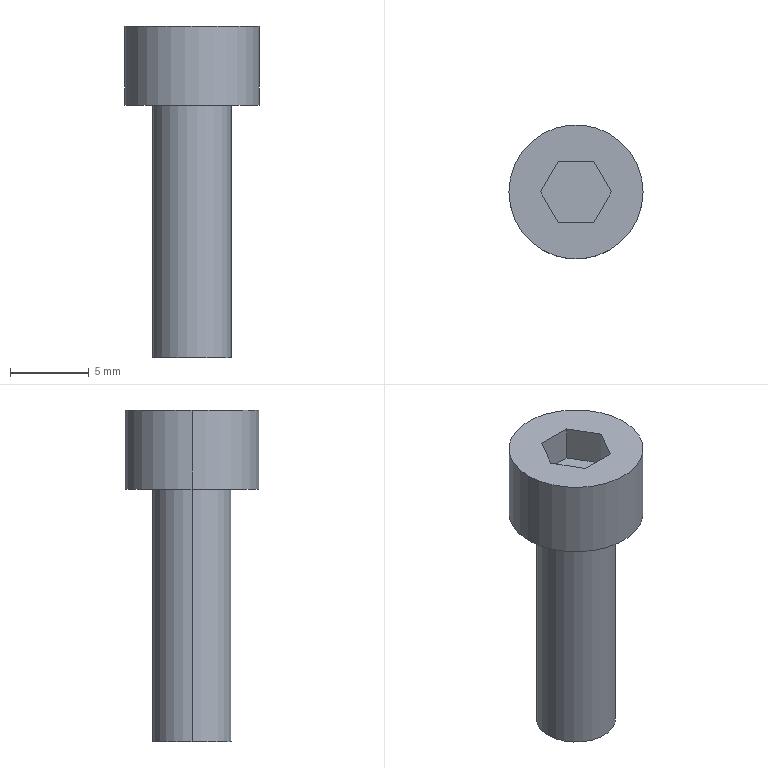Part | SolidWorks | features BaseBody 1 | 1 solid | 14 faces | box 8.5 x 8.5 x 21 mm | volume 568.291 mm3 | plane 10 | cylinder 4 | commonest cylinder face diameters 5 x2 8.5 x2
STEP:
#1=CARTESIAN_POINT('',(2.5,0.,-16.));
#2=VERTEX_POINT('',#1);
#3=CARTESIAN_POINT('',(-2.5,0.,-16.));
#4=VERTEX_POINT('',#3);
#5=CARTESIAN_POINT('',(0.,0.,-16.));
#6=DIRECTION('',(0.,0.,1.));
#7=DIRECTION('',(1.,0.,0.));
#8=AXIS2_PLACEMENT_3D('',#5,#6,#7);
#9=CIRCLE('',#8,2.5);
#10=EDGE_CURVE('',#2,#4,#9,.T.);
#11=ORIENTED_EDGE('',*,*,#10,.T.);
#12=CARTESIAN_POINT('',(-2.5,0.,0.));
#13=VERTEX_POINT('',#12);
#14=CARTESIAN_POINT('',(-2.5,0.,-16.));
#15=DIRECTION('',(0.,0.,1.));
#16=VECTOR('',#15,1000.);
#17=LINE('',#14,#16);
#18=EDGE_CURVE('',#4,#13,#17,.T.);
#19=ORIENTED_EDGE('',*,*,#18,.T.);
#20=CARTESIAN_POINT('',(2.5,0.,0.));
#21=VERTEX_POINT('',#20);
#22=CARTESIAN_POINT('',(0.,0.,0.));
#23=DIRECTION('',(0.,0.,-1.));
#24=DIRECTION('',(1.,0.,0.));
#25=AXIS2_PLACEMENT_3D('',#22,#23,#24);
#26=CIRCLE('',#25,2.5);
#27=EDGE_CURVE('',#13,#21,#26,.T.);
#28=ORIENTED_EDGE('',*,*,#27,.T.);
#29=CARTESIAN_POINT('',(2.5,0.,-16.));
#30=DIRECTION('',(0.,0.,1.));
#31=VECTOR('',#30,1000.);
#32=LINE('',#29,#31);
#33=EDGE_CURVE('',#2,#21,#32,.T.);
#34=ORIENTED_EDGE('',*,*,#33,.F.);
#35=EDGE_LOOP('',(#11,#19,#28,#34));
#36=FACE_OUTER_BOUND('',#35,.T.);
#37=CARTESIAN_POINT('',(0.,0.,-16.));
#38=DIRECTION('',(0.,0.,1.));
#39=DIRECTION('',(1.,0.,0.));
#40=AXIS2_PLACEMENT_3D('',#37,#38,#39);
#41=CYLINDRICAL_SURFACE('',#40,2.5);
#42=ADVANCED_FACE('',(#36),#41,.T.);
#43=CARTESIAN_POINT('',(4.25,0.,0.));
#44=VERTEX_POINT('',#43);
#45=CARTESIAN_POINT('',(-4.25,0.,0.));
#46=VERTEX_POINT('',#45);
#47=CARTESIAN_POINT('',(0.,0.,0.));
#48=DIRECTION('',(0.,0.,1.));
#49=DIRECTION('',(1.,0.,0.));
#50=AXIS2_PLACEMENT_3D('',#47,#48,#49);
#51=CIRCLE('',#50,4.25);
#52=EDGE_CURVE('',#44,#46,#51,.T.);
#53=ORIENTED_EDGE('',*,*,#52,.T.);
#54=CARTESIAN_POINT('',(-4.25,0.,5.));
#55=VERTEX_POINT('',#54);
#56=CARTESIAN_POINT('',(-4.25,0.,0.));
#57=DIRECTION('',(0.,0.,1.));
#58=VECTOR('',#57,1000.);
#59=LINE('',#56,#58);
#60=EDGE_CURVE('',#46,#55,#59,.T.);
#61=ORIENTED_EDGE('',*,*,#60,.T.);
#62=CARTESIAN_POINT('',(4.25,0.,5.));
#63=VERTEX_POINT('',#62);
#64=CARTESIAN_POINT('',(0.,0.,5.));
#65=DIRECTION('',(0.,0.,-1.));
#66=DIRECTION('',(1.,0.,0.));
#67=AXIS2_PLACEMENT_3D('',#64,#65,#66);
#68=CIRCLE('',#67,4.25);
#69=EDGE_CURVE('',#55,#63,#68,.T.);
#70=ORIENTED_EDGE('',*,*,#69,.T.);
#71=CARTESIAN_POINT('',(4.25,0.,0.));
#72=DIRECTION('',(0.,0.,1.));
#73=VECTOR('',#72,1000.);
#74=LINE('',#71,#73);
#75=EDGE_CURVE('',#44,#63,#74,.T.);
#76=ORIENTED_EDGE('',*,*,#75,.F.);
#77=EDGE_LOOP('',(#53,#61,#70,#76));
#78=FACE_OUTER_BOUND('',#77,.T.);
#79=CARTESIAN_POINT('',(0.,0.,0.));
#80=DIRECTION('',(0.,0.,1.));
#81=DIRECTION('',(1.,0.,0.));
#82=AXIS2_PLACEMENT_3D('',#79,#80,#81);
#83=CYLINDRICAL_SURFACE('',#82,4.25);
#84=ADVANCED_FACE('',(#78),#83,.T.);
#85=ORIENTED_EDGE('',*,*,#18,.F.);
#86=CARTESIAN_POINT('',(0.,0.,-16.));
#87=DIRECTION('',(0.,0.,1.));
#88=DIRECTION('',(1.,0.,0.));
#89=AXIS2_PLACEMENT_3D('',#86,#87,#88);
#90=CIRCLE('',#89,2.5);
#91=EDGE_CURVE('',#4,#2,#90,.T.);
#92=ORIENTED_EDGE('',*,*,#91,.T.);
#93=ORIENTED_EDGE('',*,*,#33,.T.);
#94=CARTESIAN_POINT('',(0.,0.,0.));
#95=DIRECTION('',(0.,0.,-1.));
#96=DIRECTION('',(1.,0.,0.));
#97=AXIS2_PLACEMENT_3D('',#94,#95,#96);
#98=CIRCLE('',#97,2.5);
#99=EDGE_CURVE('',#21,#13,#98,.T.);
#100=ORIENTED_EDGE('',*,*,#99,.T.);
#101=EDGE_LOOP('',(#85,#92,#93,#100));
#102=FACE_OUTER_BOUND('',#101,.T.);
#103=CARTESIAN_POINT('',(0.,0.,-16.));
#104=DIRECTION('',(0.,0.,1.));
#105=DIRECTION('',(1.,0.,0.));
#106=AXIS2_PLACEMENT_3D('',#103,#104,#105);
#107=CYLINDRICAL_SURFACE('',#106,2.5);
#108=ADVANCED_FACE('',(#102),#107,.T.);
#109=ORIENTED_EDGE('',*,*,#10,.F.);
#110=ORIENTED_EDGE('',*,*,#91,.F.);
#111=EDGE_LOOP('',(#109,#110));
#112=FACE_OUTER_BOUND('',#111,.T.);
#113=CARTESIAN_POINT('',(0.,0.,-16.));
#114=DIRECTION('',(0.,0.,1.));
#115=DIRECTION('',(1.,0.,0.));
#116=AXIS2_PLACEMENT_3D('',#113,#114,#115);
#117=PLANE('',#116);
#118=ADVANCED_FACE('',(#112),#117,.F.);
#119=ORIENTED_EDGE('',*,*,#99,.F.);
#120=ORIENTED_EDGE('',*,*,#27,.F.);
#121=EDGE_LOOP('',(#119,#120));
#122=FACE_BOUND('',#121,.T.);
#123=ORIENTED_EDGE('',*,*,#52,.F.);
#124=CARTESIAN_POINT('',(0.,0.,0.));
#125=DIRECTION('',(0.,0.,1.));
#126=DIRECTION('',(1.,0.,0.));
#127=AXIS2_PLACEMENT_3D('',#124,#125,#126);
#128=CIRCLE('',#127,4.25);
#129=EDGE_CURVE('',#46,#44,#128,.T.);
#130=ORIENTED_EDGE('',*,*,#129,.F.);
#131=EDGE_LOOP('',(#123,#130));
#132=FACE_OUTER_BOUND('',#131,.T.);
#133=CARTESIAN_POINT('',(0.,0.,0.));
#134=DIRECTION('',(0.,0.,1.));
#135=DIRECTION('',(1.,0.,0.));
#136=AXIS2_PLACEMENT_3D('',#133,#134,#135);
#137=PLANE('',#136);
#138=ADVANCED_FACE('',(#122,#132),#137,.F.);
#139=ORIENTED_EDGE('',*,*,#60,.F.);
#140=ORIENTED_EDGE('',*,*,#129,.T.);
#141=ORIENTED_EDGE('',*,*,#75,.T.);
#142=CARTESIAN_POINT('',(0.,0.,5.));
#143=DIRECTION('',(0.,0.,-1.));
#144=DIRECTION('',(1.,0.,0.));
#145=AXIS2_PLACEMENT_3D('',#142,#143,#144);
#146=CIRCLE('',#145,4.25);
#147=EDGE_CURVE('',#63,#55,#146,.T.);
#148=ORIENTED_EDGE('',*,*,#147,.T.);
#149=EDGE_LOOP('',(#139,#140,#141,#148));
#150=FACE_OUTER_BOUND('',#149,.T.);
#151=CARTESIAN_POINT('',(0.,0.,0.));
#152=DIRECTION('',(0.,0.,1.));
#153=DIRECTION('',(1.,0.,0.));
#154=AXIS2_PLACEMENT_3D('',#151,#152,#153);
#155=CYLINDRICAL_SURFACE('',#154,4.25);
#156=ADVANCED_FACE('',(#150),#155,.T.);
#157=CARTESIAN_POINT('',(-1.125,-1.949,5.));
#158=VERTEX_POINT('',#157);
#159=CARTESIAN_POINT('',(-2.25,0.,5.));
#160=VERTEX_POINT('',#159);
#161=CARTESIAN_POINT('',(-1.125,-1.949,5.));
#162=DIRECTION('',(-0.5,0.866,0.));
#163=VECTOR('',#162,1000.);
#164=LINE('',#161,#163);
#165=EDGE_CURVE('',#158,#160,#164,.T.);
#166=ORIENTED_EDGE('',*,*,#165,.T.);
#167=CARTESIAN_POINT('',(-1.125,1.949,5.));
#168=VERTEX_POINT('',#167);
#169=CARTESIAN_POINT('',(-2.25,0.,5.));
#170=DIRECTION('',(0.5,0.866,0.));
#171=VECTOR('',#170,1000.);
#172=LINE('',#169,#171);
#173=EDGE_CURVE('',#160,#168,#172,.T.);
#174=ORIENTED_EDGE('',*,*,#173,.T.);
#175=CARTESIAN_POINT('',(1.125,1.949,5.));
#176=VERTEX_POINT('',#175);
#177=CARTESIAN_POINT('',(0.,1.949,5.));
#178=DIRECTION('',(1.,0.,0.));
#179=VECTOR('',#178,1000.);
#180=LINE('',#177,#179);
#181=EDGE_CURVE('',#168,#176,#180,.T.);
#182=ORIENTED_EDGE('',*,*,#181,.T.);
#183=CARTESIAN_POINT('',(2.25,0.,5.));
#184=VERTEX_POINT('',#183);
#185=CARTESIAN_POINT('',(1.125,1.949,5.));
#186=DIRECTION('',(0.5,-0.866,0.));
#187=VECTOR('',#186,1000.);
#188=LINE('',#185,#187);
#189=EDGE_CURVE('',#176,#184,#188,.T.);
#190=ORIENTED_EDGE('',*,*,#189,.T.);
#191=CARTESIAN_POINT('',(1.125,-1.949,5.));
#192=VERTEX_POINT('',#191);
#193=CARTESIAN_POINT('',(2.25,0.,5.));
#194=DIRECTION('',(-0.5,-0.866,0.));
#195=VECTOR('',#194,1000.);
#196=LINE('',#193,#195);
#197=EDGE_CURVE('',#184,#192,#196,.T.);
#198=ORIENTED_EDGE('',*,*,#197,.T.);
#199=CARTESIAN_POINT('',(0.,-1.949,5.));
#200=DIRECTION('',(-1.,0.,0.));
#201=VECTOR('',#200,1000.);
#202=LINE('',#199,#201);
#203=EDGE_CURVE('',#192,#158,#202,.T.);
#204=ORIENTED_EDGE('',*,*,#203,.T.);
#205=EDGE_LOOP('',(#166,#174,#182,#190,#198,#204));
#206=FACE_BOUND('',#205,.T.);
#207=ORIENTED_EDGE('',*,*,#147,.F.);
#208=ORIENTED_EDGE('',*,*,#69,.F.);
#209=EDGE_LOOP('',(#207,#208));
#210=FACE_OUTER_BOUND('',#209,.T.);
#211=CARTESIAN_POINT('',(0.,0.,5.));
#212=DIRECTION('',(0.,0.,1.));
#213=DIRECTION('',(1.,0.,0.));
#214=AXIS2_PLACEMENT_3D('',#211,#212,#213);
#215=PLANE('',#214);
#216=ADVANCED_FACE('',(#206,#210),#215,.T.);
#217=ORIENTED_EDGE('',*,*,#173,.F.);
#218=CARTESIAN_POINT('',(-2.25,0.,2.75));
#219=VERTEX_POINT('',#218);
#220=CARTESIAN_POINT('',(-2.25,0.,2.75));
#221=DIRECTION('',(0.,0.,-1.));
#222=VECTOR('',#221,1000.);
#223=LINE('',#220,#222);
#224=EDGE_CURVE('',#160,#219,#223,.T.);
#225=ORIENTED_EDGE('',*,*,#224,.T.);
#226=CARTESIAN_POINT('',(-1.125,1.949,2.75));
#227=VERTEX_POINT('',#226);
#228=CARTESIAN_POINT('',(-1.125,1.949,2.75));
#229=DIRECTION('',(0.5,0.866,0.));
#230=VECTOR('',#229,1000.);
#231=LINE('',#228,#230);
#232=EDGE_CURVE('',#219,#227,#231,.T.);
#233=ORIENTED_EDGE('',*,*,#232,.T.);
#234=CARTESIAN_POINT('',(-1.125,1.949,2.75));
#235=DIRECTION('',(0.,0.,1.));
#236=VECTOR('',#235,1000.);
#237=LINE('',#234,#236);
#238=EDGE_CURVE('',#227,#168,#237,.T.);
#239=ORIENTED_EDGE('',*,*,#238,.T.);
#240=EDGE_LOOP('',(#217,#225,#233,#239));
#241=FACE_OUTER_BOUND('',#240,.T.);
#242=CARTESIAN_POINT('',(-1.125,1.949,2.75));
#243=DIRECTION('',(0.866,-0.5,0.));
#244=DIRECTION('',(0.5,0.866,0.));
#245=AXIS2_PLACEMENT_3D('',#242,#243,#244);
#246=PLANE('',#245);
#247=ADVANCED_FACE('',(#241),#246,.T.);
#248=ORIENTED_EDGE('',*,*,#165,.F.);
#249=CARTESIAN_POINT('',(-1.125,-1.949,2.75));
#250=VERTEX_POINT('',#249);
#251=CARTESIAN_POINT('',(-1.125,-1.949,2.75));
#252=DIRECTION('',(0.,0.,-1.));
#253=VECTOR('',#252,1000.);
#254=LINE('',#251,#253);
#255=EDGE_CURVE('',#158,#250,#254,.T.);
#256=ORIENTED_EDGE('',*,*,#255,.T.);
#257=CARTESIAN_POINT('',(-2.25,0.,2.75));
#258=DIRECTION('',(-0.5,0.866,0.));
#259=VECTOR('',#258,1000.);
#260=LINE('',#257,#259);
#261=EDGE_CURVE('',#250,#219,#260,.T.);
#262=ORIENTED_EDGE('',*,*,#261,.T.);
#263=ORIENTED_EDGE('',*,*,#224,.F.);
#264=EDGE_LOOP('',(#248,#256,#262,#263));
#265=FACE_OUTER_BOUND('',#264,.T.);
#266=CARTESIAN_POINT('',(-2.25,0.,2.75));
#267=DIRECTION('',(0.866,0.5,0.));
#268=DIRECTION('',(-0.5,0.866,0.));
#269=AXIS2_PLACEMENT_3D('',#266,#267,#268);
#270=PLANE('',#269);
#271=ADVANCED_FACE('',(#265),#270,.T.);
#272=ORIENTED_EDGE('',*,*,#203,.F.);
#273=CARTESIAN_POINT('',(1.125,-1.949,2.75));
#274=VERTEX_POINT('',#273);
#275=CARTESIAN_POINT('',(1.125,-1.949,2.75));
#276=DIRECTION('',(0.,0.,-1.));
#277=VECTOR('',#276,1000.);
#278=LINE('',#275,#277);
#279=EDGE_CURVE('',#192,#274,#278,.T.);
#280=ORIENTED_EDGE('',*,*,#279,.T.);
#281=CARTESIAN_POINT('',(-1.125,-1.949,2.75));
#282=DIRECTION('',(-1.,0.,0.));
#283=VECTOR('',#282,1000.);
#284=LINE('',#281,#283);
#285=EDGE_CURVE('',#274,#250,#284,.T.);
#286=ORIENTED_EDGE('',*,*,#285,.T.);
#287=ORIENTED_EDGE('',*,*,#255,.F.);
#288=EDGE_LOOP('',(#272,#280,#286,#287));
#289=FACE_OUTER_BOUND('',#288,.T.);
#290=CARTESIAN_POINT('',(-1.125,-1.949,2.75));
#291=DIRECTION('',(0.,1.,0.));
#292=DIRECTION('',(-1.,0.,0.));
#293=AXIS2_PLACEMENT_3D('',#290,#291,#292);
#294=PLANE('',#293);
#295=ADVANCED_FACE('',(#289),#294,.T.);
#296=ORIENTED_EDGE('',*,*,#197,.F.);
#297=CARTESIAN_POINT('',(2.25,0.,2.75));
#298=VERTEX_POINT('',#297);
#299=CARTESIAN_POINT('',(2.25,0.,2.75));
#300=DIRECTION('',(0.,0.,-1.));
#301=VECTOR('',#300,1000.);
#302=LINE('',#299,#301);
#303=EDGE_CURVE('',#184,#298,#302,.T.);
#304=ORIENTED_EDGE('',*,*,#303,.T.);
#305=CARTESIAN_POINT('',(1.125,-1.949,2.75));
#306=DIRECTION('',(-0.5,-0.866,0.));
#307=VECTOR('',#306,1000.);
#308=LINE('',#305,#307);
#309=EDGE_CURVE('',#298,#274,#308,.T.);
#310=ORIENTED_EDGE('',*,*,#309,.T.);
#311=ORIENTED_EDGE('',*,*,#279,.F.);
#312=EDGE_LOOP('',(#296,#304,#310,#311));
#313=FACE_OUTER_BOUND('',#312,.T.);
#314=CARTESIAN_POINT('',(1.125,-1.949,2.75));
#315=DIRECTION('',(-0.866,0.5,0.));
#316=DIRECTION('',(-0.5,-0.866,0.));
#317=AXIS2_PLACEMENT_3D('',#314,#315,#316);
#318=PLANE('',#317);
#319=ADVANCED_FACE('',(#313),#318,.T.);
#320=ORIENTED_EDGE('',*,*,#189,.F.);
#321=CARTESIAN_POINT('',(1.125,1.949,2.75));
#322=VERTEX_POINT('',#321);
#323=CARTESIAN_POINT('',(1.125,1.949,2.75));
#324=DIRECTION('',(0.,0.,-1.));
#325=VECTOR('',#324,1000.);
#326=LINE('',#323,#325);
#327=EDGE_CURVE('',#176,#322,#326,.T.);
#328=ORIENTED_EDGE('',*,*,#327,.T.);
#329=CARTESIAN_POINT('',(2.25,0.,2.75));
#330=DIRECTION('',(0.5,-0.866,0.));
#331=VECTOR('',#330,1000.);
#332=LINE('',#329,#331);
#333=EDGE_CURVE('',#322,#298,#332,.T.);
#334=ORIENTED_EDGE('',*,*,#333,.T.);
#335=ORIENTED_EDGE('',*,*,#303,.F.);
#336=EDGE_LOOP('',(#320,#328,#334,#335));
#337=FACE_OUTER_BOUND('',#336,.T.);
#338=CARTESIAN_POINT('',(2.25,0.,2.75));
#339=DIRECTION('',(-0.866,-0.5,0.));
#340=DIRECTION('',(0.5,-0.866,0.));
#341=AXIS2_PLACEMENT_3D('',#338,#339,#340);
#342=PLANE('',#341);
#343=ADVANCED_FACE('',(#337),#342,.T.);
#344=ORIENTED_EDGE('',*,*,#181,.F.);
#345=ORIENTED_EDGE('',*,*,#238,.F.);
#346=CARTESIAN_POINT('',(1.125,1.949,2.75));
#347=DIRECTION('',(1.,0.,0.));
#348=VECTOR('',#347,1000.);
#349=LINE('',#346,#348);
#350=EDGE_CURVE('',#227,#322,#349,.T.);
#351=ORIENTED_EDGE('',*,*,#350,.T.);
#352=ORIENTED_EDGE('',*,*,#327,.F.);
#353=EDGE_LOOP('',(#344,#345,#351,#352));
#354=FACE_OUTER_BOUND('',#353,.T.);
#355=CARTESIAN_POINT('',(1.125,1.949,2.75));
#356=DIRECTION('',(0.,-1.,0.));
#357=DIRECTION('',(1.,0.,0.));
#358=AXIS2_PLACEMENT_3D('',#355,#356,#357);
#359=PLANE('',#358);
#360=ADVANCED_FACE('',(#354),#359,.T.);
#361=ORIENTED_EDGE('',*,*,#285,.F.);
#362=ORIENTED_EDGE('',*,*,#309,.F.);
#363=ORIENTED_EDGE('',*,*,#333,.F.);
#364=ORIENTED_EDGE('',*,*,#350,.F.);
#365=ORIENTED_EDGE('',*,*,#232,.F.);
#366=ORIENTED_EDGE('',*,*,#261,.F.);
#367=EDGE_LOOP('',(#361,#362,#363,#364,#365,#366));
#368=FACE_OUTER_BOUND('',#367,.T.);
#369=CARTESIAN_POINT('',(0.,0.,2.75));
#370=DIRECTION('',(0.,0.,1.));
#371=DIRECTION('',(1.,0.,0.));
#372=AXIS2_PLACEMENT_3D('',#369,#370,#371);
#373=PLANE('',#372);
#374=ADVANCED_FACE('',(#368),#373,.T.);
#375=CLOSED_SHELL('',(#42,#84,#108,#118,#138,#156,#216,#247,#271,#295,#319,#343,#360,#374));
#376=MANIFOLD_SOLID_BREP('',#375);
#377=CARTESIAN_POINT('',(0.,0.,0.));
#378=DIRECTION('',(0.,0.,1.));
#379=DIRECTION('',(1.,0.,0.));
#380=AXIS2_PLACEMENT_3D('',#377,#378,#379);
#381=(LENGTH_UNIT()NAMED_UNIT(*)SI_UNIT(.MILLI.,.METRE.));
#382=UNCERTAINTY_MEASURE_WITH_UNIT(LENGTH_MEASURE(0.00001),#381,'','');
#383=(NAMED_UNIT(*)PLANE_ANGLE_UNIT()SI_UNIT($,.RADIAN.));
#384=(NAMED_UNIT(*)SI_UNIT($,.STERADIAN.)SOLID_ANGLE_UNIT());
#385=(GEOMETRIC_REPRESENTATION_CONTEXT(3)GLOBAL_UNCERTAINTY_ASSIGNED_CONTEXT((#382))GLOBAL_UNIT_ASSIGNED_CONTEXT((#381,#383,#384))REPRESENTATION_CONTEXT('',''));
#386=ADVANCED_BREP_SHAPE_REPRESENTATION('',(#376,#380),#385);